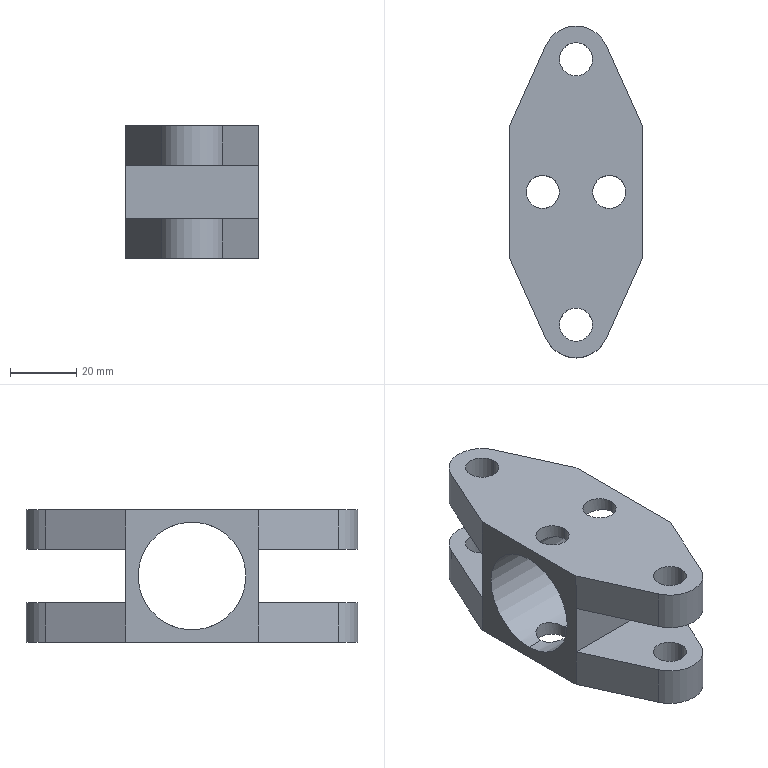Part | SolidWorks | features MirrorStock 1 | 1 solid | 40 faces | box 40 x 100 x 40 mm | volume 63212 mm3 | cylinder 22 | plane 18 | commonest cylinder face diameters 10 x16 20 x4 32.5 x2